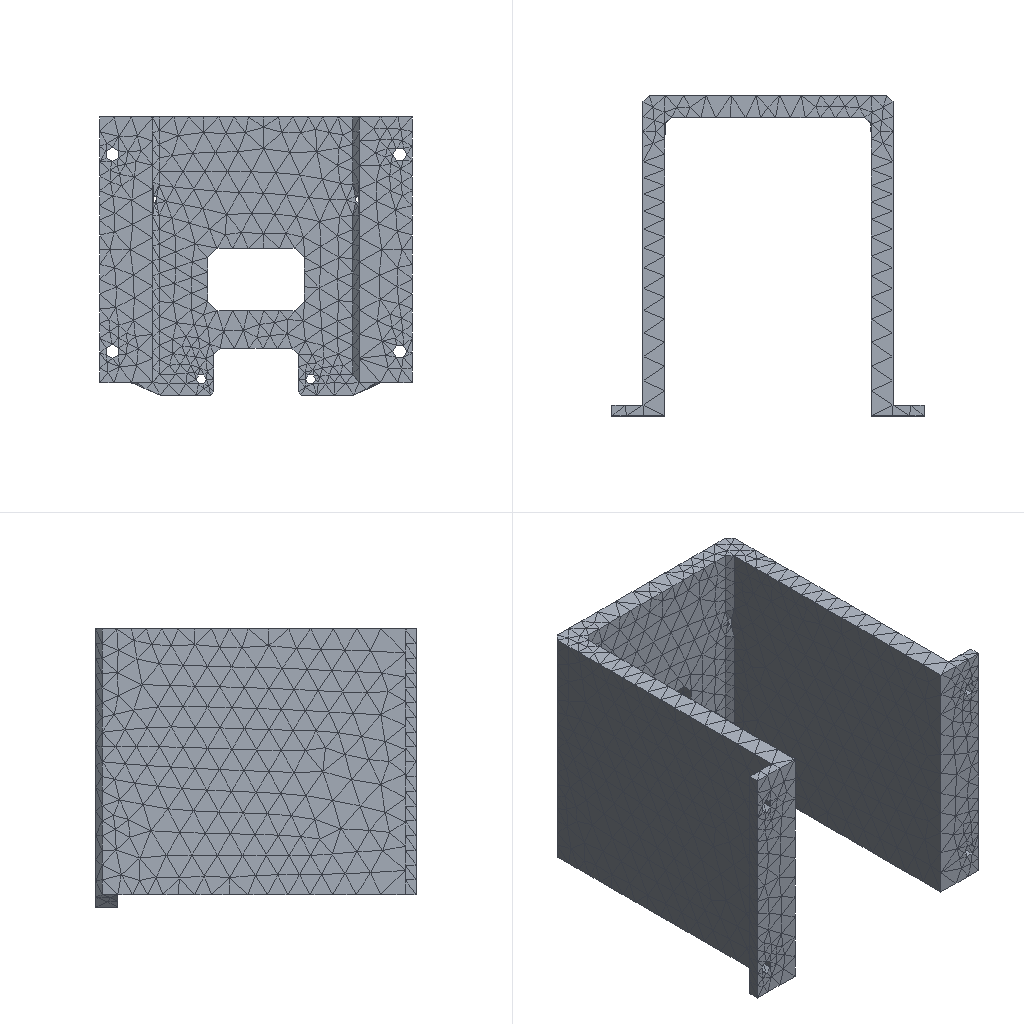Simulation study | nx simcenter
Set-up summary:
category,name,step,type,value,unit,region
solver,nx_nastran (Simcenter)
units,not stated in the deck,,not stated
analysis,deck,,static,static
analysis,solution,,SOL,101
load_step,SUBCASE 1,1,SUBCASE,SPC=1 LOAD=2
load_step,requested,,,1
mesh,nodes,,,10470
mesh,elements,,,5076
element_type,CTETRA,,solid,5076
load,nodal force total,,FX,0.0,model units
load,nodal force total,,FY,-2304999.96,model units
load,nodal force total,,FZ,0.0,model units
load,load commands in deck,,count,940
bc,support commands in deck,,count,596
analysis,NX solution 0,,Structural,Linear Statics - Single Constraint
check,setup vs results,,match,every grid point's frame and coordinates and every element id; grid points of CTETRA elements
Nastran input file, long lists of numbers shortened:
$*$$$$$$$$$$$$$$$$$$$$$$$$$$$$$$$$$$$$$$$$$$$$$$$$$$$$$$$$$$$$$$$$$
$*
$*                    NX v10.0.0.24 TRANSLATOR
$*                    FOR NX NASTRAN VERSION 10.0
$ (33 more lines like these left out)
ASSIGN OUTPUT2='129_sim1-solution_1.op2' UNIT=12
$*
$*$$$$$$$$$$$$$$$$$$$$$$$$$$$$$$$$$$$
$*
$* EXECUTIVE CONTROL
$*
$*$$$$$$$$$$$$$$$$$$$$$$$$$$$$$$$$$$$
$*
ID,NASTRAN,129_sim1-solution_1
SOL 101
CEND
$*
$*$$$$$$$$$$$$$$$$$$$$$$$$$$$$$$$$$$$
$*
$* CASE CONTROL
$*
$*$$$$$$$$$$$$$$$$$$$$$$$$$$$$$$$$$$$
$*
TITLE = Solution 1
ECHO = NONE
SPC = 1
OUTPUT
BCRESULTS(TRACTION,FORCE,PLOT) = ALL
DISPLACEMENT(PLOT) = ALL
ESE(PLOT) = ALL
FORCE(PLOT,CORNER) = ALL
OLOAD(PLOT) = ALL
SPCFORCES(PLOT) = ALL
STRAIN(PLOT,FIBER,CORNER) = ALL
STRESS(PLOT,CORNER) = ALL
$*  NX Step: Subcase - Static Loads 1
SUBCASE 1
LABEL = Subcase - Static Loads 1
LOAD = 2
$*
$*$$$$$$$$$$$$$$$$$$$$$$$$$$$$$$$$$$$
$*
$* BULK DATA
$*
$*$$$$$$$$$$$$$$$$$$$$$$$$$$$$$$$$$$$
$*
BEGIN BULK
$*
$* PARAM CARDS
$*
PARAM      K6ROT100.0000
PARAM     OIBULK     YES
PARAM    OMACHPR     YES
PARAM       POST      -2
PARAM    POSTEXT     YES
PARAM    UNITSYS   MN-MM
$*
$* GRID CARDS
$*
GRID*              10375               0-9.000000000E+01-1.025000000E+02+
*       8.5000000000E+01               0
GRID*              10376               0-9.000000000E+01-1.025000000E+02+
*       0.0000000000E+00               0
$ (20936 more lines like these left out)
$*
$* ELEMENT CARDS
$*
$*  NX Mesh Collector: Solid(1)
$*  NX Mesh: 3d_mesh(1)
CTETRA         1       1       1    3731    9386       2      73    3922+
+             74      75      76      77
CTETRA         2       1       2    3731    9386    9387      76    3922+
+             77      78    3927    9395
$ (10148 more lines like these left out)
$*
$* PROPERTY CARDS
$*
$*  NX Property: PSOLID1
PSOLID         1       1       0                           SMECH
$*
$* MATERIAL CARDS
$*
$*  NX Material: Aluminum_6061
MAT1           16.8980+7        0.3300002.7110-62.2161-5
MATT1          1       1               2               3
TABLEM1        1                                                        +
+        20.00006.8980+7 21.11006.8980+7 23.89006.8980+7 37.78006.8290+7+
+        51.67006.8290+7 65.56006.7600+7 79.44006.6910+7 93.33006.6221+7+
+       107.22006.5531+7121.11006.4841+7135.00006.4151+7148.89006.3461+7+
+       162.78006.2772+7176.67006.1392+7190.56006.0702+7204.44005.9323+7+
+       218.33005.8633+7232.22005.7253+7246.11005.5874+7260.00005.4494+7+
+       273.89005.3114+7287.78005.1735+7301.67005.0355+7315.56004.8976+7+
+       329.44004.7596+7343.33004.6216+7357.22004.4147+7371.11004.2767+7+
+       385.00004.1388+7398.89003.9318+7412.78003.7939+7426.67003.5869+7+
+           ENDT
TABLEM1        2                                                        +
+        20.00000.330000 21.11000.330000    ENDT
TABLEM1        3                                                        +
+        20.00002.2380-5 93.33002.3184-5107.22002.3346-5121.11002.3508-5+
+       135.00002.3670-5148.89002.3832-5162.78002.3994-5176.67002.4138-5+
+       190.56002.4300-5204.44002.4444-5218.33002.4588-5232.22002.4732-5+
+       246.11002.4876-5260.00002.5002-5273.89002.5146-5287.78002.5272-5+
+       301.67002.5398-5315.56002.5524-5    ENDT
$*
$* LOAD AND CONSTRAINT CARDS
$*
$*  NX Load and Constraint: Fixed(1)
SPC            1    3490  123456  0.0000
SPC            1    3491  123456  0.0000
SPC            1    3492  123456  0.0000
SPC            1    3493  123456  0.0000
$ (592 more lines like these left out)
$*  NX Load and Constraint: Force(1)
FORCE          2    7409       0 3561.30  0.0000-1.00000  0.0000
FORCE          2    7410       0 3732.18  0.0000-1.00000  0.0000
FORCE          2    7411       0 3156.47  0.0000-1.00000  0.0000
FORCE          2    7412       0 2760.80  0.0000-1.00000  0.0000
$ (936 more lines like these left out)
ENDDATA a1d66759
Results summary:
result,analysis,,,static
result,last_loadstep,,,1
result,primary field,,,displacements
result,max displacement,,,0.04153,model units
result,reaction total,,FX,0.01348,model units
result,reaction total,,FY,2305000.0,model units
result,reaction total,,FZ,-0.01057,model units
result,NX solution 0,,loadcases,1,mm